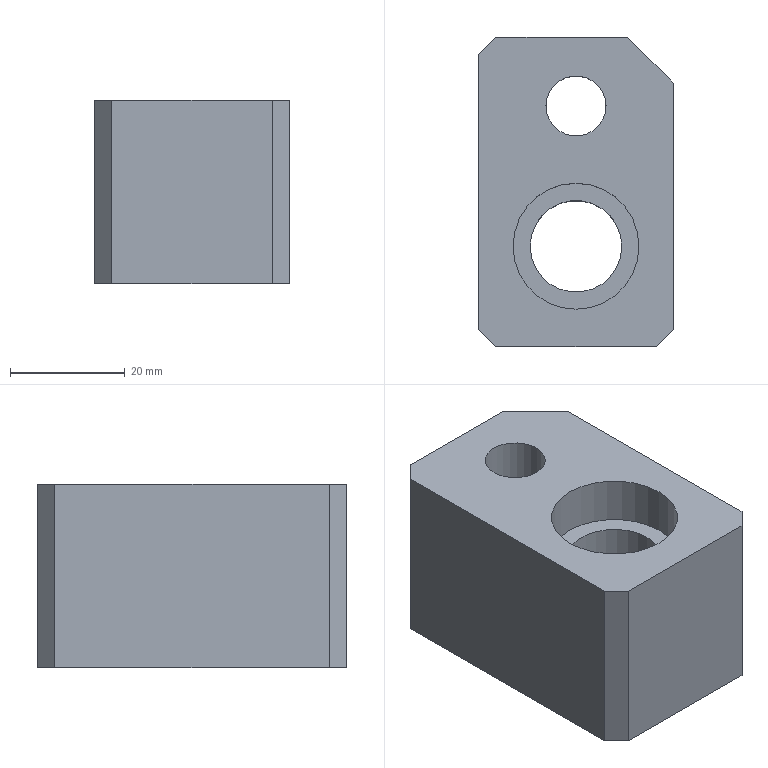Part | STEP file | lll_id3562_x_t | 1 solid | 16 faces | box 34 x 54 x 32 mm | volume 44236 mm3 | plane 12 | cylinder 4 | commonest cylinder face diameters 10.5 x1 16 x1 17 x1 22 x1
STEP:
#1=CARTESIAN_POINT('',(3682.5,-59.5,60.5));
#2=VERTEX_POINT('',#1);
#3=CARTESIAN_POINT('',(3690.5,-59.5,60.5));
#4=DIRECTION('',(0.,0.,1.));
#5=DIRECTION('',(-1.,0.,0.));
#6=AXIS2_PLACEMENT_3D('',#3,#4,#5);
#7=CIRCLE('',#6,8.);
#8=EDGE_CURVE('',#2,#2,#7,.T.);
#9=ORIENTED_EDGE('',*,*,#8,.T.);
#10=EDGE_LOOP('',(#9));
#11=FACE_BOUND('',#10,.T.);
#12=CARTESIAN_POINT('',(3704.5,-77.,60.5));
#13=VERTEX_POINT('',#12);
#14=CARTESIAN_POINT('',(3676.5,-77.,60.5));
#15=VERTEX_POINT('',#14);
#16=CARTESIAN_POINT('',(3690.5,-77.,60.5));
#17=DIRECTION('',(-1.,0.,0.));
#18=VECTOR('',#17,1.);
#19=LINE('',#16,#18);
#20=EDGE_CURVE('',#13,#15,#19,.T.);
#21=ORIENTED_EDGE('',*,*,#20,.T.);
#22=CARTESIAN_POINT('',(3673.5,-74.,60.5));
#23=VERTEX_POINT('',#22);
#24=CARTESIAN_POINT('',(3673.5,-74.,60.5));
#25=DIRECTION('',(-0.7071,0.7071,0.));
#26=VECTOR('',#25,1.);
#27=LINE('',#24,#26);
#28=EDGE_CURVE('',#15,#23,#27,.T.);
#29=ORIENTED_EDGE('',*,*,#28,.T.);
#30=CARTESIAN_POINT('',(3673.5,-26.,60.5));
#31=VERTEX_POINT('',#30);
#32=CARTESIAN_POINT('',(3673.5,-28.275,60.5));
#33=DIRECTION('',(0.,1.,0.));
#34=VECTOR('',#33,1.);
#35=LINE('',#32,#34);
#36=EDGE_CURVE('',#23,#31,#35,.T.);
#37=ORIENTED_EDGE('',*,*,#36,.T.);
#38=CARTESIAN_POINT('',(3676.5,-23.,60.5));
#39=VERTEX_POINT('',#38);
#40=CARTESIAN_POINT('',(3676.5,-23.,60.5));
#41=DIRECTION('',(-0.7071,-0.7071,0.));
#42=VECTOR('',#41,1.);
#43=LINE('',#40,#42);
#44=EDGE_CURVE('',#39,#31,#43,.T.);
#45=ORIENTED_EDGE('',*,*,#44,.F.);
#46=CARTESIAN_POINT('',(3699.5,-23.,60.5));
#47=VERTEX_POINT('',#46);
#48=CARTESIAN_POINT('',(3690.5,-23.,60.5));
#49=DIRECTION('',(1.,0.,0.));
#50=VECTOR('',#49,1.);
#51=LINE('',#48,#50);
#52=EDGE_CURVE('',#39,#47,#51,.T.);
#53=ORIENTED_EDGE('',*,*,#52,.T.);
#54=CARTESIAN_POINT('',(3707.5,-31.,60.5));
#55=VERTEX_POINT('',#54);
#56=CARTESIAN_POINT('',(3699.5,-23.,60.5));
#57=DIRECTION('',(-0.7071,0.7071,0.));
#58=VECTOR('',#57,1.);
#59=LINE('',#56,#58);
#60=EDGE_CURVE('',#55,#47,#59,.T.);
#61=ORIENTED_EDGE('',*,*,#60,.F.);
#62=CARTESIAN_POINT('',(3707.5,-74.,60.5));
#63=VERTEX_POINT('',#62);
#64=CARTESIAN_POINT('',(3707.5,-28.275,60.5));
#65=DIRECTION('',(0.,-1.,0.));
#66=VECTOR('',#65,1.);
#67=LINE('',#64,#66);
#68=EDGE_CURVE('',#55,#63,#67,.T.);
#69=ORIENTED_EDGE('',*,*,#68,.T.);
#70=CARTESIAN_POINT('',(3704.5,-77.,60.5));
#71=DIRECTION('',(0.7071,0.7071,0.));
#72=VECTOR('',#71,1.);
#73=LINE('',#70,#72);
#74=EDGE_CURVE('',#13,#63,#73,.T.);
#75=ORIENTED_EDGE('',*,*,#74,.F.);
#76=EDGE_LOOP('',(#21,#29,#37,#45,#53,#61,#69,#75));
#77=FACE_BOUND('',#76,.T.);
#78=CARTESIAN_POINT('',(3682.,-35.,60.5));
#79=VERTEX_POINT('',#78);
#80=CARTESIAN_POINT('',(3690.5,-35.,60.5));
#81=DIRECTION('',(0.,0.,-1.));
#82=DIRECTION('',(-1.,0.,0.));
#83=AXIS2_PLACEMENT_3D('',#80,#81,#82);
#84=CIRCLE('',#83,8.5);
#85=EDGE_CURVE('',#79,#79,#84,.T.);
#86=ORIENTED_EDGE('',*,*,#85,.F.);
#87=EDGE_LOOP('',(#86));
#88=FACE_BOUND('',#87,.T.);
#89=CARTESIAN_POINT('',(3622.36,-28.275,60.5));
#90=DIRECTION('',(0.,0.,1.));
#91=DIRECTION('',(-1.,0.,0.));
#92=AXIS2_PLACEMENT_3D('',#89,#90,#91);
#93=PLANE('',#92);
#94=ADVANCED_FACE('',(#11,#77,#88),#93,.F.);
#95=CARTESIAN_POINT('',(3679.5,-59.5,92.5));
#96=VERTEX_POINT('',#95);
#97=CARTESIAN_POINT('',(3690.5,-59.5,92.5));
#98=DIRECTION('',(0.,0.,-1.));
#99=DIRECTION('',(-1.,0.,0.));
#100=AXIS2_PLACEMENT_3D('',#97,#98,#99);
#101=CIRCLE('',#100,11.);
#102=EDGE_CURVE('',#96,#96,#101,.T.);
#103=ORIENTED_EDGE('',*,*,#102,.T.);
#104=EDGE_LOOP('',(#103));
#105=FACE_BOUND('',#104,.T.);
#106=CARTESIAN_POINT('',(3685.25,-35.,92.5));
#107=VERTEX_POINT('',#106);
#108=CARTESIAN_POINT('',(3690.5,-35.,92.5));
#109=DIRECTION('',(0.,0.,-1.));
#110=DIRECTION('',(-1.,0.,0.));
#111=AXIS2_PLACEMENT_3D('',#108,#109,#110);
#112=CIRCLE('',#111,5.25);
#113=EDGE_CURVE('',#107,#107,#112,.T.);
#114=ORIENTED_EDGE('',*,*,#113,.T.);
#115=EDGE_LOOP('',(#114));
#116=FACE_BOUND('',#115,.T.);
#117=CARTESIAN_POINT('',(3673.5,-26.,92.5));
#118=VERTEX_POINT('',#117);
#119=CARTESIAN_POINT('',(3673.5,-74.,92.5));
#120=VERTEX_POINT('',#119);
#121=CARTESIAN_POINT('',(3673.5,-28.275,92.5));
#122=DIRECTION('',(0.,-1.,0.));
#123=VECTOR('',#122,1.);
#124=LINE('',#121,#123);
#125=EDGE_CURVE('',#118,#120,#124,.T.);
#126=ORIENTED_EDGE('',*,*,#125,.T.);
#127=CARTESIAN_POINT('',(3676.5,-77.,92.5));
#128=VERTEX_POINT('',#127);
#129=CARTESIAN_POINT('',(3625.067,-25.567,92.5));
#130=DIRECTION('',(0.7071,-0.7071,0.));
#131=VECTOR('',#130,1.);
#132=LINE('',#129,#131);
#133=EDGE_CURVE('',#120,#128,#132,.T.);
#134=ORIENTED_EDGE('',*,*,#133,.T.);
#135=CARTESIAN_POINT('',(3704.5,-77.,92.5));
#136=VERTEX_POINT('',#135);
#137=CARTESIAN_POINT('',(3690.5,-77.,92.5));
#138=DIRECTION('',(1.,0.,0.));
#139=VECTOR('',#138,1.);
#140=LINE('',#137,#139);
#141=EDGE_CURVE('',#128,#136,#140,.T.);
#142=ORIENTED_EDGE('',*,*,#141,.T.);
#143=CARTESIAN_POINT('',(3707.5,-74.,92.5));
#144=VERTEX_POINT('',#143);
#145=CARTESIAN_POINT('',(3704.5,-77.,92.5));
#146=DIRECTION('',(-0.7071,-0.7071,0.));
#147=VECTOR('',#146,1.);
#148=LINE('',#145,#147);
#149=EDGE_CURVE('',#144,#136,#148,.T.);
#150=ORIENTED_EDGE('',*,*,#149,.F.);
#151=CARTESIAN_POINT('',(3707.5,-31.,92.5));
#152=VERTEX_POINT('',#151);
#153=CARTESIAN_POINT('',(3707.5,-28.275,92.5));
#154=DIRECTION('',(0.,1.,0.));
#155=VECTOR('',#154,1.);
#156=LINE('',#153,#155);
#157=EDGE_CURVE('',#144,#152,#156,.T.);
#158=ORIENTED_EDGE('',*,*,#157,.T.);
#159=CARTESIAN_POINT('',(3699.5,-23.,92.5));
#160=VERTEX_POINT('',#159);
#161=CARTESIAN_POINT('',(3699.5,-23.,92.5));
#162=DIRECTION('',(0.7071,-0.7071,0.));
#163=VECTOR('',#162,1.);
#164=LINE('',#161,#163);
#165=EDGE_CURVE('',#160,#152,#164,.T.);
#166=ORIENTED_EDGE('',*,*,#165,.F.);
#167=CARTESIAN_POINT('',(3676.5,-23.,92.5));
#168=VERTEX_POINT('',#167);
#169=CARTESIAN_POINT('',(3690.5,-23.,92.5));
#170=DIRECTION('',(-1.,0.,0.));
#171=VECTOR('',#170,1.);
#172=LINE('',#169,#171);
#173=EDGE_CURVE('',#160,#168,#172,.T.);
#174=ORIENTED_EDGE('',*,*,#173,.T.);
#175=CARTESIAN_POINT('',(3676.5,-23.,92.5));
#176=DIRECTION('',(0.7071,0.7071,0.));
#177=VECTOR('',#176,1.);
#178=LINE('',#175,#177);
#179=EDGE_CURVE('',#118,#168,#178,.T.);
#180=ORIENTED_EDGE('',*,*,#179,.F.);
#181=EDGE_LOOP('',(#126,#134,#142,#150,#158,#166,#174,#180));
#182=FACE_BOUND('',#181,.T.);
#183=CARTESIAN_POINT('',(3622.36,-28.275,92.5));
#184=DIRECTION('',(0.,0.,1.));
#185=DIRECTION('',(-1.,0.,0.));
#186=AXIS2_PLACEMENT_3D('',#183,#184,#185);
#187=PLANE('',#186);
#188=ADVANCED_FACE('',(#105,#116,#182),#187,.T.);
#189=ORIENTED_EDGE('',*,*,#141,.F.);
#190=CARTESIAN_POINT('',(3676.5,-77.,-8.5));
#191=DIRECTION('',(0.,0.,-1.));
#192=VECTOR('',#191,1.);
#193=LINE('',#190,#192);
#194=EDGE_CURVE('',#128,#15,#193,.T.);
#195=ORIENTED_EDGE('',*,*,#194,.T.);
#196=ORIENTED_EDGE('',*,*,#20,.F.);
#197=CARTESIAN_POINT('',(3704.5,-77.,-8.5));
#198=DIRECTION('',(0.,0.,-1.));
#199=VECTOR('',#198,1.);
#200=LINE('',#197,#199);
#201=EDGE_CURVE('',#136,#13,#200,.T.);
#202=ORIENTED_EDGE('',*,*,#201,.F.);
#203=EDGE_LOOP('',(#189,#195,#196,#202));
#204=FACE_OUTER_BOUND('',#203,.T.);
#205=CARTESIAN_POINT('',(3690.5,-77.,-8.5));
#206=DIRECTION('',(0.,-1.,0.));
#207=DIRECTION('',(0.,0.,-1.));
#208=AXIS2_PLACEMENT_3D('',#205,#206,#207);
#209=PLANE('',#208);
#210=ADVANCED_FACE('',(#204),#209,.T.);
#211=ORIENTED_EDGE('',*,*,#157,.F.);
#212=CARTESIAN_POINT('',(3707.5,-74.,-8.5));
#213=DIRECTION('',(0.,0.,1.));
#214=VECTOR('',#213,1.);
#215=LINE('',#212,#214);
#216=EDGE_CURVE('',#63,#144,#215,.T.);
#217=ORIENTED_EDGE('',*,*,#216,.F.);
#218=ORIENTED_EDGE('',*,*,#68,.F.);
#219=CARTESIAN_POINT('',(3707.5,-31.,-8.5));
#220=DIRECTION('',(0.,0.,-1.));
#221=VECTOR('',#220,1.);
#222=LINE('',#219,#221);
#223=EDGE_CURVE('',#152,#55,#222,.T.);
#224=ORIENTED_EDGE('',*,*,#223,.F.);
#225=EDGE_LOOP('',(#211,#217,#218,#224));
#226=FACE_OUTER_BOUND('',#225,.T.);
#227=CARTESIAN_POINT('',(3707.5,-59.5,-8.5));
#228=DIRECTION('',(1.,0.,0.));
#229=DIRECTION('',(0.,0.,1.));
#230=AXIS2_PLACEMENT_3D('',#227,#228,#229);
#231=PLANE('',#230);
#232=ADVANCED_FACE('',(#226),#231,.T.);
#233=ORIENTED_EDGE('',*,*,#52,.F.);
#234=CARTESIAN_POINT('',(3676.5,-23.,-8.5));
#235=DIRECTION('',(0.,0.,-1.));
#236=VECTOR('',#235,1.);
#237=LINE('',#234,#236);
#238=EDGE_CURVE('',#168,#39,#237,.T.);
#239=ORIENTED_EDGE('',*,*,#238,.F.);
#240=ORIENTED_EDGE('',*,*,#173,.F.);
#241=CARTESIAN_POINT('',(3699.5,-23.,-8.5));
#242=DIRECTION('',(0.,0.,1.));
#243=VECTOR('',#242,1.);
#244=LINE('',#241,#243);
#245=EDGE_CURVE('',#47,#160,#244,.T.);
#246=ORIENTED_EDGE('',*,*,#245,.F.);
#247=EDGE_LOOP('',(#233,#239,#240,#246));
#248=FACE_OUTER_BOUND('',#247,.T.);
#249=CARTESIAN_POINT('',(3690.5,-23.,-8.5));
#250=DIRECTION('',(0.,1.,0.));
#251=DIRECTION('',(0.,0.,1.));
#252=AXIS2_PLACEMENT_3D('',#249,#250,#251);
#253=PLANE('',#252);
#254=ADVANCED_FACE('',(#248),#253,.T.);
#255=ORIENTED_EDGE('',*,*,#36,.F.);
#256=CARTESIAN_POINT('',(3673.5,-74.,-8.5));
#257=DIRECTION('',(0.,0.,1.));
#258=VECTOR('',#257,1.);
#259=LINE('',#256,#258);
#260=EDGE_CURVE('',#23,#120,#259,.T.);
#261=ORIENTED_EDGE('',*,*,#260,.T.);
#262=ORIENTED_EDGE('',*,*,#125,.F.);
#263=CARTESIAN_POINT('',(3673.5,-26.,-8.5));
#264=DIRECTION('',(0.,0.,1.));
#265=VECTOR('',#264,1.);
#266=LINE('',#263,#265);
#267=EDGE_CURVE('',#31,#118,#266,.T.);
#268=ORIENTED_EDGE('',*,*,#267,.F.);
#269=EDGE_LOOP('',(#255,#261,#262,#268));
#270=FACE_OUTER_BOUND('',#269,.T.);
#271=CARTESIAN_POINT('',(3673.5,-59.5,-8.5));
#272=DIRECTION('',(-1.,0.,0.));
#273=DIRECTION('',(0.,0.,-1.));
#274=AXIS2_PLACEMENT_3D('',#271,#272,#273);
#275=PLANE('',#274);
#276=ADVANCED_FACE('',(#270),#275,.T.);
#277=ORIENTED_EDGE('',*,*,#113,.F.);
#278=EDGE_LOOP('',(#277));
#279=FACE_BOUND('',#278,.T.);
#280=CARTESIAN_POINT('',(3685.25,-35.,77.5));
#281=VERTEX_POINT('',#280);
#282=CARTESIAN_POINT('',(3690.5,-35.,77.5));
#283=DIRECTION('',(0.,0.,1.));
#284=DIRECTION('',(-1.,0.,0.));
#285=AXIS2_PLACEMENT_3D('',#282,#283,#284);
#286=CIRCLE('',#285,5.25);
#287=EDGE_CURVE('',#281,#281,#286,.T.);
#288=ORIENTED_EDGE('',*,*,#287,.F.);
#289=EDGE_LOOP('',(#288));
#290=FACE_BOUND('',#289,.T.);
#291=CARTESIAN_POINT('',(3690.5,-35.,160.5));
#292=DIRECTION('',(0.,0.,1.));
#293=DIRECTION('',(-1.,0.,0.));
#294=AXIS2_PLACEMENT_3D('',#291,#292,#293);
#295=CYLINDRICAL_SURFACE('',#294,5.25);
#296=ADVANCED_FACE('',(#279,#290),#295,.F.);
#297=ORIENTED_EDGE('',*,*,#287,.T.);
#298=EDGE_LOOP('',(#297));
#299=FACE_BOUND('',#298,.T.);
#300=CARTESIAN_POINT('',(3682.,-35.,77.5));
#301=VERTEX_POINT('',#300);
#302=CARTESIAN_POINT('',(3690.5,-35.,77.5));
#303=DIRECTION('',(0.,0.,1.));
#304=DIRECTION('',(-1.,0.,0.));
#305=AXIS2_PLACEMENT_3D('',#302,#303,#304);
#306=CIRCLE('',#305,8.5);
#307=EDGE_CURVE('',#301,#301,#306,.T.);
#308=ORIENTED_EDGE('',*,*,#307,.F.);
#309=EDGE_LOOP('',(#308));
#310=FACE_BOUND('',#309,.T.);
#311=CARTESIAN_POINT('',(3690.5,-35.,77.5));
#312=DIRECTION('',(0.,0.,1.));
#313=DIRECTION('',(-1.,0.,0.));
#314=AXIS2_PLACEMENT_3D('',#311,#312,#313);
#315=PLANE('',#314);
#316=ADVANCED_FACE('',(#299,#310),#315,.F.);
#317=ORIENTED_EDGE('',*,*,#307,.T.);
#318=EDGE_LOOP('',(#317));
#319=FACE_BOUND('',#318,.T.);
#320=ORIENTED_EDGE('',*,*,#85,.T.);
#321=EDGE_LOOP('',(#320));
#322=FACE_BOUND('',#321,.T.);
#323=CARTESIAN_POINT('',(3690.5,-35.,60.5));
#324=DIRECTION('',(0.,0.,1.));
#325=DIRECTION('',(-1.,0.,0.));
#326=AXIS2_PLACEMENT_3D('',#323,#324,#325);
#327=CYLINDRICAL_SURFACE('',#326,8.5);
#328=ADVANCED_FACE('',(#319,#322),#327,.F.);
#329=ORIENTED_EDGE('',*,*,#102,.F.);
#330=EDGE_LOOP('',(#329));
#331=FACE_BOUND('',#330,.T.);
#332=CARTESIAN_POINT('',(3701.5,-59.5,84.3));
#333=VERTEX_POINT('',#332);
#334=CARTESIAN_POINT('',(3690.5,-59.5,84.3));
#335=DIRECTION('',(0.,0.,1.));
#336=DIRECTION('',(1.,0.,0.));
#337=AXIS2_PLACEMENT_3D('',#334,#335,#336);
#338=CIRCLE('',#337,11.);
#339=EDGE_CURVE('',#333,#333,#338,.T.);
#340=ORIENTED_EDGE('',*,*,#339,.F.);
#341=EDGE_LOOP('',(#340));
#342=FACE_BOUND('',#341,.T.);
#343=CARTESIAN_POINT('',(3690.5,-59.5,90.));
#344=DIRECTION('',(0.,0.,-1.));
#345=DIRECTION('',(0.,-1.,0.));
#346=AXIS2_PLACEMENT_3D('',#343,#344,#345);
#347=CYLINDRICAL_SURFACE('',#346,11.);
#348=ADVANCED_FACE('',(#331,#342),#347,.F.);
#349=ORIENTED_EDGE('',*,*,#339,.T.);
#350=EDGE_LOOP('',(#349));
#351=FACE_BOUND('',#350,.T.);
#352=CARTESIAN_POINT('',(3698.5,-59.5,84.3));
#353=VERTEX_POINT('',#352);
#354=CARTESIAN_POINT('',(3690.5,-59.5,84.3));
#355=DIRECTION('',(0.,0.,1.));
#356=DIRECTION('',(1.,0.,0.));
#357=AXIS2_PLACEMENT_3D('',#354,#355,#356);
#358=CIRCLE('',#357,8.);
#359=EDGE_CURVE('',#353,#353,#358,.T.);
#360=ORIENTED_EDGE('',*,*,#359,.F.);
#361=EDGE_LOOP('',(#360));
#362=FACE_BOUND('',#361,.T.);
#363=CARTESIAN_POINT('',(3690.5,-50.75,84.3));
#364=DIRECTION('',(0.,0.,-1.));
#365=DIRECTION('',(0.,1.,0.));
#366=AXIS2_PLACEMENT_3D('',#363,#364,#365);
#367=PLANE('',#366);
#368=ADVANCED_FACE('',(#351,#362),#367,.F.);
#369=ORIENTED_EDGE('',*,*,#8,.F.);
#370=EDGE_LOOP('',(#369));
#371=FACE_BOUND('',#370,.T.);
#372=ORIENTED_EDGE('',*,*,#359,.T.);
#373=EDGE_LOOP('',(#372));
#374=FACE_BOUND('',#373,.T.);
#375=CARTESIAN_POINT('',(3690.5,-59.5,44.8));
#376=DIRECTION('',(0.,0.,-1.));
#377=DIRECTION('',(0.,-1.,0.));
#378=AXIS2_PLACEMENT_3D('',#375,#376,#377);
#379=CYLINDRICAL_SURFACE('',#378,8.);
#380=ADVANCED_FACE('',(#371,#374),#379,.F.);
#381=ORIENTED_EDGE('',*,*,#179,.T.);
#382=ORIENTED_EDGE('',*,*,#238,.T.);
#383=ORIENTED_EDGE('',*,*,#44,.T.);
#384=ORIENTED_EDGE('',*,*,#267,.T.);
#385=EDGE_LOOP('',(#381,#382,#383,#384));
#386=FACE_OUTER_BOUND('',#385,.T.);
#387=CARTESIAN_POINT('',(3676.5,-23.,-8.5));
#388=DIRECTION('',(0.7071,-0.7071,0.));
#389=DIRECTION('',(0.7071,0.7071,0.));
#390=AXIS2_PLACEMENT_3D('',#387,#388,#389);
#391=PLANE('',#390);
#392=ADVANCED_FACE('',(#386),#391,.F.);
#393=ORIENTED_EDGE('',*,*,#149,.T.);
#394=ORIENTED_EDGE('',*,*,#201,.T.);
#395=ORIENTED_EDGE('',*,*,#74,.T.);
#396=ORIENTED_EDGE('',*,*,#216,.T.);
#397=EDGE_LOOP('',(#393,#394,#395,#396));
#398=FACE_OUTER_BOUND('',#397,.T.);
#399=CARTESIAN_POINT('',(3704.5,-77.,-8.5));
#400=DIRECTION('',(-0.7071,0.7071,0.));
#401=DIRECTION('',(-0.7071,-0.7071,0.));
#402=AXIS2_PLACEMENT_3D('',#399,#400,#401);
#403=PLANE('',#402);
#404=ADVANCED_FACE('',(#398),#403,.F.);
#405=ORIENTED_EDGE('',*,*,#60,.T.);
#406=ORIENTED_EDGE('',*,*,#245,.T.);
#407=ORIENTED_EDGE('',*,*,#165,.T.);
#408=ORIENTED_EDGE('',*,*,#223,.T.);
#409=EDGE_LOOP('',(#405,#406,#407,#408));
#410=FACE_OUTER_BOUND('',#409,.T.);
#411=CARTESIAN_POINT('',(3699.5,-23.,-8.5));
#412=DIRECTION('',(-0.7071,-0.7071,0.));
#413=DIRECTION('',(0.7071,-0.7071,0.));
#414=AXIS2_PLACEMENT_3D('',#411,#412,#413);
#415=PLANE('',#414);
#416=ADVANCED_FACE('',(#410),#415,.F.);
#417=ORIENTED_EDGE('',*,*,#28,.F.);
#418=ORIENTED_EDGE('',*,*,#194,.F.);
#419=ORIENTED_EDGE('',*,*,#133,.F.);
#420=ORIENTED_EDGE('',*,*,#260,.F.);
#421=EDGE_LOOP('',(#417,#418,#419,#420));
#422=FACE_OUTER_BOUND('',#421,.T.);
#423=CARTESIAN_POINT('',(3673.5,-74.,-8.5));
#424=DIRECTION('',(0.7071,0.7071,0.));
#425=DIRECTION('',(0.,0.,1.));
#426=AXIS2_PLACEMENT_3D('',#423,#424,#425);
#427=PLANE('',#426);
#428=ADVANCED_FACE('',(#422),#427,.F.);
#429=CLOSED_SHELL('',(#94,#188,#210,#232,#254,#276,#296,#316,#328,#348,#368,#380,#392,#404,#416,#428));
#430=MANIFOLD_SOLID_BREP('',#429);
#431=(LENGTH_UNIT()NAMED_UNIT(*)SI_UNIT(.MILLI.,.METRE.));
#432=UNCERTAINTY_MEASURE_WITH_UNIT(LENGTH_MEASURE(0.00002),#431,'','');
#433=(NAMED_UNIT(*)PLANE_ANGLE_UNIT()SI_UNIT($,.RADIAN.));
#434=PLANE_ANGLE_MEASURE_WITH_UNIT(PLANE_ANGLE_MEASURE(0.01745),#433);
#435=DIMENSIONAL_EXPONENTS(0.,0.,0.,0.,0.,0.,0.);
#436=(CONVERSION_BASED_UNIT('DEGREE',#434)NAMED_UNIT(#435)PLANE_ANGLE_UNIT());
#437=(NAMED_UNIT(*)SI_UNIT($,.STERADIAN.)SOLID_ANGLE_UNIT());
#438=(GEOMETRIC_REPRESENTATION_CONTEXT(3)GLOBAL_UNCERTAINTY_ASSIGNED_CONTEXT((#432))GLOBAL_UNIT_ASSIGNED_CONTEXT((#431,#436,#437))REPRESENTATION_CONTEXT('',''));
#439=ADVANCED_BREP_SHAPE_REPRESENTATION('',(#430),#438);